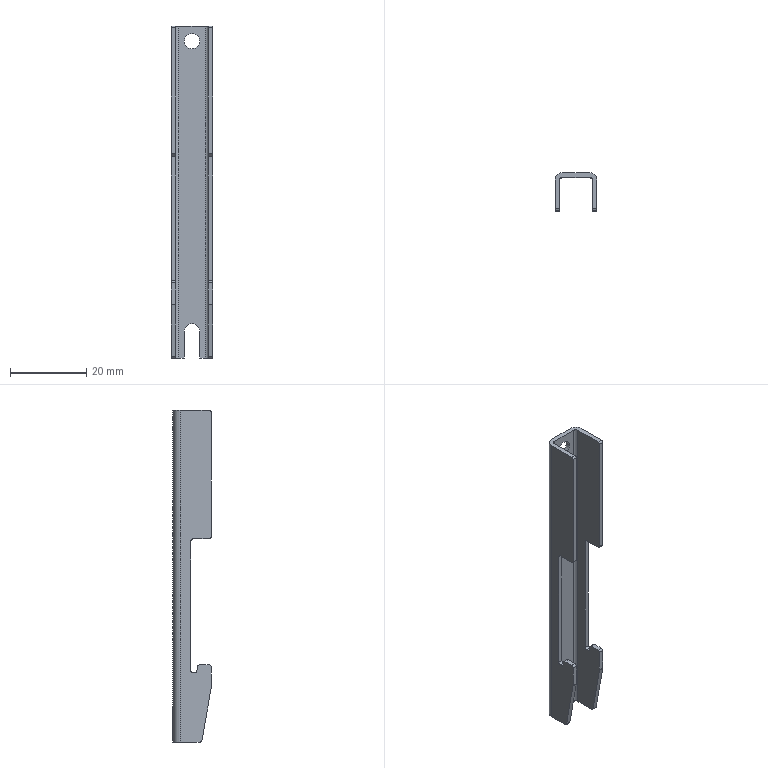Part | STEP file | SS5V1-16S3AD-08B-N1_Rail Clamp | 1 solid | 53 faces | box 11 x 10 x 87 mm | volume 2335 mm3 | plane 27 | cylinder 26 | commonest cylinder face diameters 1 x18 4 x6 1.6 x2